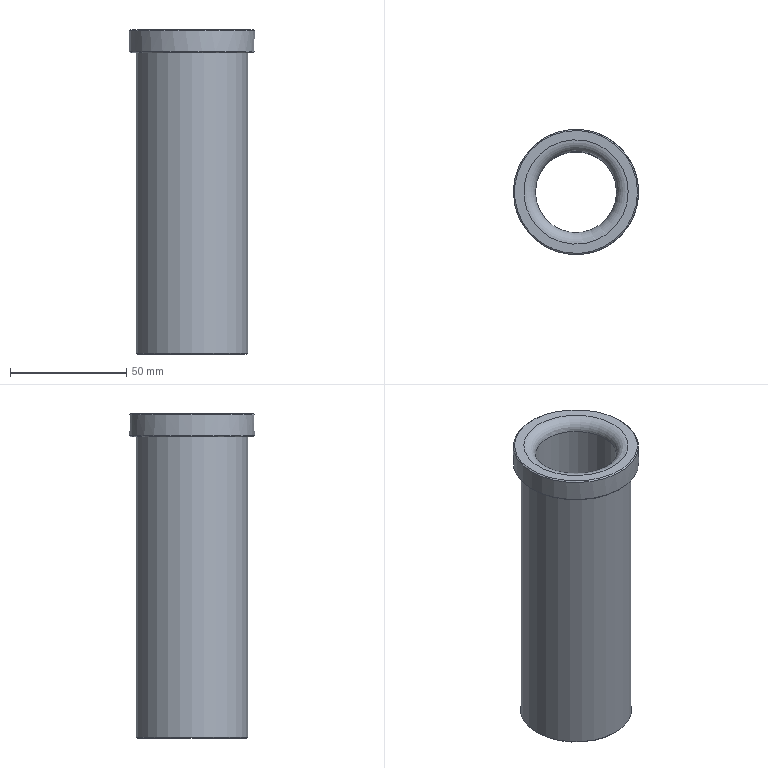Part | NX | features solid 2 | 1 solid | 11 faces | box 54 x 54 x 140 mm | volume 122133 mm3 | plane 3 | cylinder 3 | cone 3 | torus 2 | commonest cylinder face diameters 35 x1 48 x1 54 x1
STEP:
#1=CARTESIAN_POINT('',(138.,-185.,130.5));
#2=VERTEX_POINT('',#1);
#3=CARTESIAN_POINT('',(162.,-185.,130.5));
#4=DIRECTION('',(0.,0.,-1.));
#5=DIRECTION('',(-1.,0.,0.));
#6=AXIS2_PLACEMENT_3D('',#3,#4,#5);
#7=CIRCLE('',#6,24.);
#8=EDGE_CURVE('',#2,#2,#7,.T.);
#9=ORIENTED_EDGE('',*,*,#8,.F.);
#10=EDGE_LOOP('',(#9));
#11=FACE_BOUND('',#10,.T.);
#12=CARTESIAN_POINT('',(135.5,-185.,130.5));
#13=VERTEX_POINT('',#12);
#14=CARTESIAN_POINT('',(162.,-185.,130.5));
#15=DIRECTION('',(0.,0.,-1.));
#16=DIRECTION('',(-1.,0.,0.));
#17=AXIS2_PLACEMENT_3D('',#14,#15,#16);
#18=CIRCLE('',#17,26.5);
#19=EDGE_CURVE('',#13,#13,#18,.T.);
#20=ORIENTED_EDGE('',*,*,#19,.T.);
#21=EDGE_LOOP('',(#20));
#22=FACE_BOUND('',#21,.T.);
#23=CARTESIAN_POINT('',(162.,-185.,130.5));
#24=DIRECTION('',(0.,0.,-1.));
#25=DIRECTION('',(-1.,0.,0.));
#26=AXIS2_PLACEMENT_3D('',#23,#24,#25);
#27=PLANE('',#26);
#28=ADVANCED_FACE('',(#11,#22),#27,.T.);
#29=CARTESIAN_POINT('',(188.5,-185.,140.5));
#30=VERTEX_POINT('',#29);
#31=CARTESIAN_POINT('',(162.,-185.,140.5));
#32=DIRECTION('',(0.,0.,1.));
#33=DIRECTION('',(1.,0.,0.));
#34=AXIS2_PLACEMENT_3D('',#31,#32,#33);
#35=CIRCLE('',#34,26.5);
#36=EDGE_CURVE('',#30,#30,#35,.T.);
#37=ORIENTED_EDGE('',*,*,#36,.T.);
#38=EDGE_LOOP('',(#37));
#39=FACE_BOUND('',#38,.T.);
#40=CARTESIAN_POINT('',(184.5,-185.,140.5));
#41=VERTEX_POINT('',#40);
#42=CARTESIAN_POINT('',(162.,-185.,140.5));
#43=DIRECTION('',(0.,0.,1.));
#44=DIRECTION('',(1.,0.,0.));
#45=AXIS2_PLACEMENT_3D('',#42,#43,#44);
#46=CIRCLE('',#45,22.5);
#47=EDGE_CURVE('',#41,#41,#46,.F.);
#48=ORIENTED_EDGE('',*,*,#47,.T.);
#49=EDGE_LOOP('',(#48));
#50=FACE_BOUND('',#49,.T.);
#51=CARTESIAN_POINT('',(162.,-185.,140.5));
#52=DIRECTION('',(0.,0.,1.));
#53=DIRECTION('',(1.,0.,0.));
#54=AXIS2_PLACEMENT_3D('',#51,#52,#53);
#55=PLANE('',#54);
#56=ADVANCED_FACE('',(#39,#50),#55,.T.);
#57=CARTESIAN_POINT('',(189.,-185.,140.));
#58=VERTEX_POINT('',#57);
#59=CARTESIAN_POINT('',(162.,-185.,140.));
#60=DIRECTION('',(0.,0.,1.));
#61=DIRECTION('',(1.,0.,0.));
#62=AXIS2_PLACEMENT_3D('',#59,#60,#61);
#63=CIRCLE('',#62,27.);
#64=EDGE_CURVE('',#58,#58,#63,.F.);
#65=ORIENTED_EDGE('',*,*,#64,.T.);
#66=EDGE_LOOP('',(#65));
#67=FACE_BOUND('',#66,.T.);
#68=CARTESIAN_POINT('',(135.,-185.,131.));
#69=VERTEX_POINT('',#68);
#70=CARTESIAN_POINT('',(162.,-185.,131.));
#71=DIRECTION('',(0.,0.,-1.));
#72=DIRECTION('',(-1.,0.,0.));
#73=AXIS2_PLACEMENT_3D('',#70,#71,#72);
#74=CIRCLE('',#73,27.);
#75=EDGE_CURVE('',#69,#69,#74,.F.);
#76=ORIENTED_EDGE('',*,*,#75,.T.);
#77=EDGE_LOOP('',(#76));
#78=FACE_BOUND('',#77,.T.);
#79=CARTESIAN_POINT('',(162.,-185.,140.5));
#80=DIRECTION('',(0.,0.,-1.));
#81=DIRECTION('',(-1.,0.,0.));
#82=AXIS2_PLACEMENT_3D('',#79,#80,#81);
#83=CYLINDRICAL_SURFACE('',#82,27.);
#84=ADVANCED_FACE('',(#67,#78),#83,.T.);
#85=ORIENTED_EDGE('',*,*,#36,.F.);
#86=EDGE_LOOP('',(#85));
#87=FACE_BOUND('',#86,.T.);
#88=ORIENTED_EDGE('',*,*,#64,.F.);
#89=EDGE_LOOP('',(#88));
#90=FACE_BOUND('',#89,.T.);
#91=CARTESIAN_POINT('',(162.,-185.,140.));
#92=DIRECTION('',(0.,0.,-1.));
#93=DIRECTION('',(-1.,0.,0.));
#94=AXIS2_PLACEMENT_3D('',#91,#92,#93);
#95=CONICAL_SURFACE('',#94,27.,0.7854);
#96=ADVANCED_FACE('',(#87,#90),#95,.T.);
#97=ORIENTED_EDGE('',*,*,#19,.F.);
#98=EDGE_LOOP('',(#97));
#99=FACE_BOUND('',#98,.T.);
#100=ORIENTED_EDGE('',*,*,#75,.F.);
#101=EDGE_LOOP('',(#100));
#102=FACE_BOUND('',#101,.T.);
#103=CARTESIAN_POINT('',(162.,-185.,131.));
#104=DIRECTION('',(0.,0.,1.));
#105=DIRECTION('',(1.,0.,0.));
#106=AXIS2_PLACEMENT_3D('',#103,#104,#105);
#107=CONICAL_SURFACE('',#106,27.,0.7854);
#108=ADVANCED_FACE('',(#99,#102),#107,.T.);
#109=CARTESIAN_POINT('',(139.5,-185.,0.5));
#110=VERTEX_POINT('',#109);
#111=CARTESIAN_POINT('',(162.,-185.,0.5));
#112=DIRECTION('',(0.,0.,-1.));
#113=DIRECTION('',(-1.,0.,0.));
#114=AXIS2_PLACEMENT_3D('',#111,#112,#113);
#115=CIRCLE('',#114,22.5);
#116=EDGE_CURVE('',#110,#110,#115,.F.);
#117=ORIENTED_EDGE('',*,*,#116,.T.);
#118=EDGE_LOOP('',(#117));
#119=FACE_BOUND('',#118,.T.);
#120=CARTESIAN_POINT('',(138.5,-185.,0.5));
#121=VERTEX_POINT('',#120);
#122=CARTESIAN_POINT('',(162.,-185.,0.5));
#123=DIRECTION('',(0.,0.,-1.));
#124=DIRECTION('',(-1.,0.,0.));
#125=AXIS2_PLACEMENT_3D('',#122,#123,#124);
#126=CIRCLE('',#125,23.5);
#127=EDGE_CURVE('',#121,#121,#126,.T.);
#128=ORIENTED_EDGE('',*,*,#127,.T.);
#129=EDGE_LOOP('',(#128));
#130=FACE_BOUND('',#129,.T.);
#131=CARTESIAN_POINT('',(162.,-185.,0.5));
#132=DIRECTION('',(0.,0.,-1.));
#133=DIRECTION('',(-1.,0.,0.));
#134=AXIS2_PLACEMENT_3D('',#131,#132,#133);
#135=PLANE('',#134);
#136=ADVANCED_FACE('',(#119,#130),#135,.T.);
#137=ORIENTED_EDGE('',*,*,#8,.T.);
#138=EDGE_LOOP('',(#137));
#139=FACE_BOUND('',#138,.T.);
#140=CARTESIAN_POINT('',(138.,-185.,1.));
#141=VERTEX_POINT('',#140);
#142=CARTESIAN_POINT('',(162.,-185.,1.));
#143=DIRECTION('',(0.,0.,-1.));
#144=DIRECTION('',(-1.,0.,0.));
#145=AXIS2_PLACEMENT_3D('',#142,#143,#144);
#146=CIRCLE('',#145,24.);
#147=EDGE_CURVE('',#141,#141,#146,.F.);
#148=ORIENTED_EDGE('',*,*,#147,.T.);
#149=EDGE_LOOP('',(#148));
#150=FACE_BOUND('',#149,.T.);
#151=CARTESIAN_POINT('',(162.,-185.,140.5));
#152=DIRECTION('',(0.,0.,-1.));
#153=DIRECTION('',(-1.,0.,0.));
#154=AXIS2_PLACEMENT_3D('',#151,#152,#153);
#155=CYLINDRICAL_SURFACE('',#154,24.);
#156=ADVANCED_FACE('',(#139,#150),#155,.T.);
#157=ORIENTED_EDGE('',*,*,#127,.F.);
#158=EDGE_LOOP('',(#157));
#159=FACE_BOUND('',#158,.T.);
#160=ORIENTED_EDGE('',*,*,#147,.F.);
#161=EDGE_LOOP('',(#160));
#162=FACE_BOUND('',#161,.T.);
#163=CARTESIAN_POINT('',(162.,-185.,1.));
#164=DIRECTION('',(0.,0.,1.));
#165=DIRECTION('',(1.,0.,0.));
#166=AXIS2_PLACEMENT_3D('',#163,#164,#165);
#167=CONICAL_SURFACE('',#166,24.,0.7854);
#168=ADVANCED_FACE('',(#159,#162),#167,.T.);
#169=CARTESIAN_POINT('',(179.5,-185.,135.5));
#170=VERTEX_POINT('',#169);
#171=CARTESIAN_POINT('',(162.,-185.,135.5));
#172=DIRECTION('',(0.,0.,1.));
#173=DIRECTION('',(1.,0.,0.));
#174=AXIS2_PLACEMENT_3D('',#171,#172,#173);
#175=CIRCLE('',#174,17.5);
#176=EDGE_CURVE('',#170,#170,#175,.T.);
#177=ORIENTED_EDGE('',*,*,#176,.T.);
#178=EDGE_LOOP('',(#177));
#179=FACE_BOUND('',#178,.T.);
#180=CARTESIAN_POINT('',(144.5,-185.,5.5));
#181=VERTEX_POINT('',#180);
#182=CARTESIAN_POINT('',(162.,-185.,5.5));
#183=DIRECTION('',(0.,0.,-1.));
#184=DIRECTION('',(-1.,0.,0.));
#185=AXIS2_PLACEMENT_3D('',#182,#183,#184);
#186=CIRCLE('',#185,17.5);
#187=EDGE_CURVE('',#181,#181,#186,.T.);
#188=ORIENTED_EDGE('',*,*,#187,.T.);
#189=EDGE_LOOP('',(#188));
#190=FACE_BOUND('',#189,.T.);
#191=CARTESIAN_POINT('',(162.,-185.,140.5));
#192=DIRECTION('',(0.,0.,-1.));
#193=DIRECTION('',(-1.,0.,0.));
#194=AXIS2_PLACEMENT_3D('',#191,#192,#193);
#195=CYLINDRICAL_SURFACE('',#194,17.5);
#196=ADVANCED_FACE('',(#179,#190),#195,.F.);
#197=ORIENTED_EDGE('',*,*,#176,.F.);
#198=EDGE_LOOP('',(#197));
#199=FACE_BOUND('',#198,.T.);
#200=ORIENTED_EDGE('',*,*,#47,.F.);
#201=EDGE_LOOP('',(#200));
#202=FACE_BOUND('',#201,.T.);
#203=CARTESIAN_POINT('',(162.,-185.,135.5));
#204=DIRECTION('',(0.,0.,1.));
#205=DIRECTION('',(1.,0.,0.));
#206=AXIS2_PLACEMENT_3D('',#203,#204,#205);
#207=TOROIDAL_SURFACE('',#206,22.5,5.);
#208=ADVANCED_FACE('',(#199,#202),#207,.T.);
#209=ORIENTED_EDGE('',*,*,#187,.F.);
#210=EDGE_LOOP('',(#209));
#211=FACE_BOUND('',#210,.T.);
#212=ORIENTED_EDGE('',*,*,#116,.F.);
#213=EDGE_LOOP('',(#212));
#214=FACE_BOUND('',#213,.T.);
#215=CARTESIAN_POINT('',(162.,-185.,5.5));
#216=DIRECTION('',(0.,0.,-1.));
#217=DIRECTION('',(-1.,0.,0.));
#218=AXIS2_PLACEMENT_3D('',#215,#216,#217);
#219=TOROIDAL_SURFACE('',#218,22.5,5.);
#220=ADVANCED_FACE('',(#211,#214),#219,.T.);
#221=CLOSED_SHELL('',(#28,#56,#84,#96,#108,#136,#156,#168,#196,#208,#220));
#222=MANIFOLD_SOLID_BREP('',#221);
#223=(LENGTH_UNIT()NAMED_UNIT(*)SI_UNIT(.MILLI.,.METRE.));
#224=UNCERTAINTY_MEASURE_WITH_UNIT(LENGTH_MEASURE(0.00001),#223,'','');
#225=(NAMED_UNIT(*)PLANE_ANGLE_UNIT()SI_UNIT($,.RADIAN.));
#226=(NAMED_UNIT(*)SI_UNIT($,.STERADIAN.)SOLID_ANGLE_UNIT());
#227=(GEOMETRIC_REPRESENTATION_CONTEXT(3)GLOBAL_UNCERTAINTY_ASSIGNED_CONTEXT((#224))GLOBAL_UNIT_ASSIGNED_CONTEXT((#223,#225,#226))REPRESENTATION_CONTEXT('',''));
#228=ADVANCED_BREP_SHAPE_REPRESENTATION('',(#222),#227);